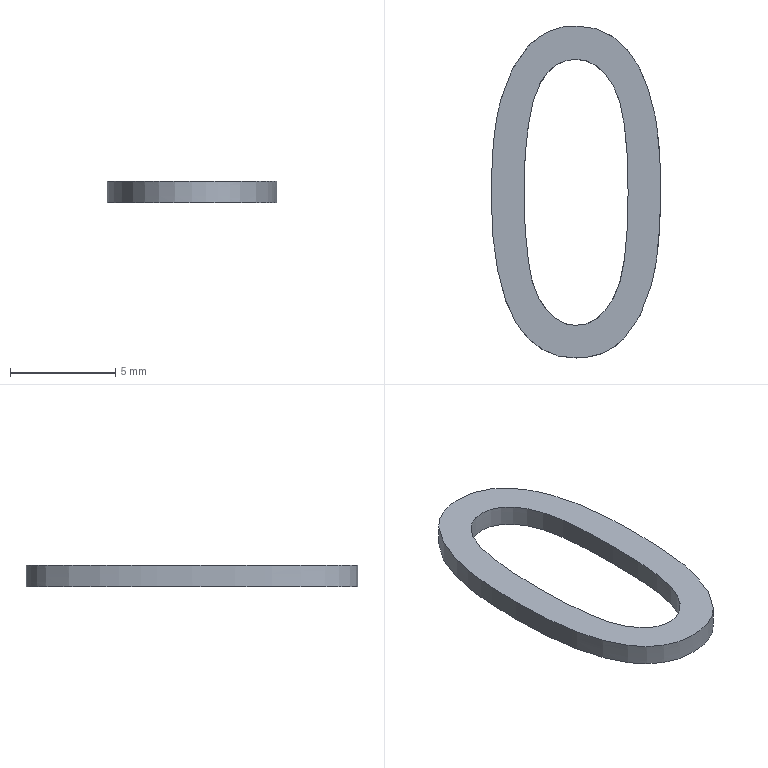Part | STEP file | lll_id966_x_t | 1 solid | 4 faces | box 8.049 x 15.752 x 1 mm | volume 54.602 mm3 | other 2 | plane 2